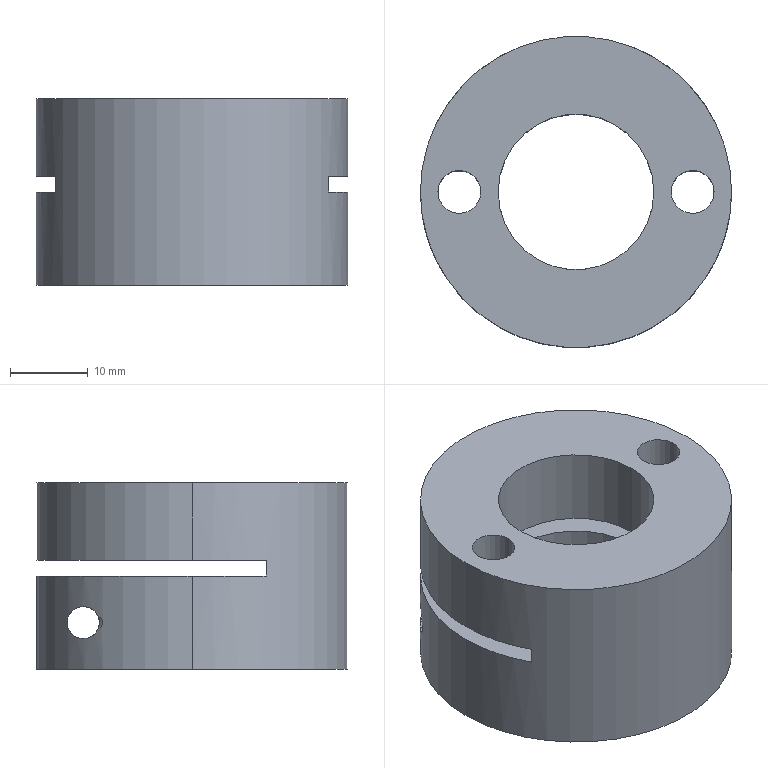Part | NX | features A0001 2 | 1 solid | 39 faces | box 40 x 40 x 24 mm | volume 19127 mm3 | cylinder 22 | plane 14 | cone 3 | commonest cylinder face diameters 5.5 x8 20 x4 40 x4 4.134 x2 5.6 x2 9 x2
STEP:
#1=CARTESIAN_POINT('',(-67.75,25.,-12.));
#2=VERTEX_POINT('',#1);
#3=CARTESIAN_POINT('',(-62.25,25.,-12.));
#4=VERTEX_POINT('',#3);
#5=CARTESIAN_POINT('',(-65.,25.,-12.));
#6=DIRECTION('',(0.,0.,-1.));
#7=DIRECTION('',(-1.,0.,0.));
#8=AXIS2_PLACEMENT_3D('',#5,#6,#7);
#9=CIRCLE('',#8,2.75);
#10=EDGE_CURVE('',#2,#4,#9,.T.);
#11=ORIENTED_EDGE('',*,*,#10,.F.);
#12=CARTESIAN_POINT('',(-67.75,25.,-22.));
#13=VERTEX_POINT('',#12);
#14=CARTESIAN_POINT('',(-67.75,25.,-22.));
#15=DIRECTION('',(0.,0.,1.));
#16=VECTOR('',#15,1000.);
#17=LINE('',#14,#16);
#18=EDGE_CURVE('',#2,#13,#17,.F.);
#19=ORIENTED_EDGE('',*,*,#18,.T.);
#20=CARTESIAN_POINT('',(-62.25,25.,-22.));
#21=VERTEX_POINT('',#20);
#22=CARTESIAN_POINT('',(-65.,25.,-22.));
#23=DIRECTION('',(0.,0.,1.));
#24=DIRECTION('',(1.,0.,0.));
#25=AXIS2_PLACEMENT_3D('',#22,#23,#24);
#26=CIRCLE('',#25,2.75);
#27=EDGE_CURVE('',#21,#13,#26,.T.);
#28=ORIENTED_EDGE('',*,*,#27,.F.);
#29=CARTESIAN_POINT('',(-62.25,25.,-22.));
#30=DIRECTION('',(0.,0.,1.));
#31=VECTOR('',#30,1000.);
#32=LINE('',#29,#31);
#33=EDGE_CURVE('',#21,#4,#32,.T.);
#34=ORIENTED_EDGE('',*,*,#33,.T.);
#35=EDGE_LOOP('',(#11,#19,#28,#34));
#36=FACE_BOUND('',#35,.T.);
#37=CARTESIAN_POINT('',(-65.,25.,-12.));
#38=DIRECTION('',(0.,0.,-1.));
#39=DIRECTION('',(-1.,0.,0.));
#40=AXIS2_PLACEMENT_3D('',#37,#38,#39);
#41=CYLINDRICAL_SURFACE('',#40,2.75);
#42=ADVANCED_FACE('',(#36),#41,.F.);
#43=ORIENTED_EDGE('',*,*,#33,.F.);
#44=CARTESIAN_POINT('',(-65.,25.,-22.));
#45=DIRECTION('',(0.,0.,1.));
#46=DIRECTION('',(-1.,0.,0.));
#47=AXIS2_PLACEMENT_3D('',#44,#45,#46);
#48=CIRCLE('',#47,2.75);
#49=EDGE_CURVE('',#13,#21,#48,.T.);
#50=ORIENTED_EDGE('',*,*,#49,.F.);
#51=ORIENTED_EDGE('',*,*,#18,.F.);
#52=CARTESIAN_POINT('',(-65.,25.,-12.));
#53=DIRECTION('',(0.,0.,-1.));
#54=DIRECTION('',(1.,0.,0.));
#55=AXIS2_PLACEMENT_3D('',#52,#53,#54);
#56=CIRCLE('',#55,2.75);
#57=EDGE_CURVE('',#4,#2,#56,.T.);
#58=ORIENTED_EDGE('',*,*,#57,.F.);
#59=EDGE_LOOP('',(#43,#50,#51,#58));
#60=FACE_BOUND('',#59,.T.);
#61=CARTESIAN_POINT('',(-65.,25.,-12.));
#62=DIRECTION('',(0.,0.,-1.));
#63=DIRECTION('',(-1.,0.,0.));
#64=AXIS2_PLACEMENT_3D('',#61,#62,#63);
#65=CYLINDRICAL_SURFACE('',#64,2.75);
#66=ADVANCED_FACE('',(#60),#65,.F.);
#67=CARTESIAN_POINT('',(-80.75,39.,-27.5));
#68=VERTEX_POINT('',#67);
#69=CARTESIAN_POINT('',(-81.183,39.,-27.933));
#70=VERTEX_POINT('',#69);
#71=CARTESIAN_POINT('',(-80.75,39.,-27.5));
#72=DIRECTION('',(-0.7071,0.,-0.7071));
#73=VECTOR('',#72,1000.);
#74=LINE('',#71,#73);
#75=EDGE_CURVE('',#68,#70,#74,.T.);
#76=ORIENTED_EDGE('',*,*,#75,.F.);
#77=CARTESIAN_POINT('',(-80.75,39.,-32.5));
#78=VERTEX_POINT('',#77);
#79=CARTESIAN_POINT('',(-80.75,39.,-30.));
#80=DIRECTION('',(-1.,0.,0.));
#81=DIRECTION('',(0.,0.,-1.));
#82=AXIS2_PLACEMENT_3D('',#79,#80,#81);
#83=CIRCLE('',#82,2.5);
#84=EDGE_CURVE('',#78,#68,#83,.T.);
#85=ORIENTED_EDGE('',*,*,#84,.F.);
#86=CARTESIAN_POINT('',(-81.183,39.,-32.067));
#87=VERTEX_POINT('',#86);
#88=CARTESIAN_POINT('',(-80.75,39.,-32.5));
#89=DIRECTION('',(-0.7071,0.,0.7071));
#90=VECTOR('',#89,1000.);
#91=LINE('',#88,#90);
#92=EDGE_CURVE('',#87,#78,#91,.F.);
#93=ORIENTED_EDGE('',*,*,#92,.F.);
#94=CARTESIAN_POINT('',(-81.183,39.,-30.));
#95=DIRECTION('',(-1.,0.,0.));
#96=DIRECTION('',(0.,0.,-1.));
#97=AXIS2_PLACEMENT_3D('',#94,#95,#96);
#98=CIRCLE('',#97,2.067);
#99=EDGE_CURVE('',#87,#70,#98,.T.);
#100=ORIENTED_EDGE('',*,*,#99,.T.);
#101=EDGE_LOOP('',(#76,#85,#93,#100));
#102=FACE_BOUND('',#101,.T.);
#103=CARTESIAN_POINT('',(-81.235,39.,-30.));
#104=DIRECTION('',(1.,0.,0.));
#105=DIRECTION('',(0.,0.,-1.));
#106=AXIS2_PLACEMENT_3D('',#103,#104,#105);
#107=CONICAL_SURFACE('',#106,2.015,0.7854);
#108=ADVANCED_FACE('',(#102),#107,.F.);
#109=CARTESIAN_POINT('',(-81.183,39.,-30.));
#110=DIRECTION('',(-1.,0.,0.));
#111=DIRECTION('',(0.,0.,1.));
#112=AXIS2_PLACEMENT_3D('',#109,#110,#111);
#113=CIRCLE('',#112,2.067);
#114=EDGE_CURVE('',#70,#87,#113,.T.);
#115=ORIENTED_EDGE('',*,*,#114,.T.);
#116=ORIENTED_EDGE('',*,*,#92,.T.);
#117=CARTESIAN_POINT('',(-80.75,39.,-30.));
#118=DIRECTION('',(-1.,0.,0.));
#119=DIRECTION('',(0.,0.,1.));
#120=AXIS2_PLACEMENT_3D('',#117,#118,#119);
#121=CIRCLE('',#120,2.5);
#122=EDGE_CURVE('',#68,#78,#121,.T.);
#123=ORIENTED_EDGE('',*,*,#122,.F.);
#124=ORIENTED_EDGE('',*,*,#75,.T.);
#125=EDGE_LOOP('',(#115,#116,#123,#124));
#126=FACE_BOUND('',#125,.T.);
#127=CARTESIAN_POINT('',(-81.235,39.,-30.));
#128=DIRECTION('',(1.,0.,0.));
#129=DIRECTION('',(0.,0.,-1.));
#130=AXIS2_PLACEMENT_3D('',#127,#128,#129);
#131=CONICAL_SURFACE('',#130,2.015,0.7854);
#132=ADVANCED_FACE('',(#126),#131,.F.);
#133=CARTESIAN_POINT('',(-94.283,39.,-32.067));
#134=VERTEX_POINT('',#133);
#135=CARTESIAN_POINT('',(-94.283,39.,-27.933));
#136=VERTEX_POINT('',#135);
#137=CARTESIAN_POINT('',(-94.283,39.,-32.067));
#138=CARTESIAN_POINT('',(-93.803,39.491,-32.067));
#139=CARTESIAN_POINT('',(-93.042,40.184,-31.817));
#140=CARTESIAN_POINT('',(-92.16,40.884,-31.003));
#141=CARTESIAN_POINT('',(-91.786,41.159,-30.));
#142=CARTESIAN_POINT('',(-92.16,40.884,-28.997));
#143=CARTESIAN_POINT('',(-93.042,40.185,-28.183));
#144=CARTESIAN_POINT('',(-93.803,39.49,-27.933));
#145=CARTESIAN_POINT('',(-94.283,39.,-27.933));
#146=B_SPLINE_CURVE_WITH_KNOTS('',3,(#137,#138,#139,#140,#141,#142,#143,#144,#145),.UNSPECIFIED.,.F.,.F.,(4,1,1,1,1,1,4),(0.,0.25,0.375,0.5,0.625,0.75,1.),.UNSPECIFIED.);
#147=EDGE_CURVE('',#134,#136,#146,.T.);
#148=ORIENTED_EDGE('',*,*,#147,.F.);
#149=CARTESIAN_POINT('',(-81.183,39.,-32.067));
#150=DIRECTION('',(-1.,0.,0.));
#151=VECTOR('',#150,1000.);
#152=LINE('',#149,#151);
#153=EDGE_CURVE('',#134,#87,#152,.F.);
#154=ORIENTED_EDGE('',*,*,#153,.T.);
#155=ORIENTED_EDGE('',*,*,#114,.F.);
#156=CARTESIAN_POINT('',(-81.183,39.,-27.933));
#157=DIRECTION('',(-1.,0.,0.));
#158=VECTOR('',#157,1000.);
#159=LINE('',#156,#158);
#160=EDGE_CURVE('',#70,#136,#159,.T.);
#161=ORIENTED_EDGE('',*,*,#160,.T.);
#162=EDGE_LOOP('',(#148,#154,#155,#161));
#163=FACE_BOUND('',#162,.T.);
#164=CARTESIAN_POINT('',(-88.557,39.,-30.));
#165=DIRECTION('',(1.,0.,0.));
#166=DIRECTION('',(0.,0.,-1.));
#167=AXIS2_PLACEMENT_3D('',#164,#165,#166);
#168=CYLINDRICAL_SURFACE('',#167,2.067);
#169=ADVANCED_FACE('',(#163),#168,.F.);
#170=CARTESIAN_POINT('',(-95.93,37.093,-30.797));
#171=VERTEX_POINT('',#170);
#172=CARTESIAN_POINT('',(-95.93,37.093,-29.203));
#173=VERTEX_POINT('',#172);
#174=CARTESIAN_POINT('',(-95.93,37.093,-30.797));
#175=CARTESIAN_POINT('',(-96.04,36.948,-30.735));
#176=CARTESIAN_POINT('',(-96.249,36.663,-30.559));
#177=CARTESIAN_POINT('',(-96.42,36.419,-30.));
#178=CARTESIAN_POINT('',(-96.249,36.663,-29.441));
#179=CARTESIAN_POINT('',(-96.04,36.948,-29.265));
#180=CARTESIAN_POINT('',(-95.93,37.093,-29.203));
#181=B_SPLINE_CURVE_WITH_KNOTS('',3,(#174,#175,#176,#177,#178,#179,#180),.UNSPECIFIED.,.F.,.F.,(4,1,1,1,4),(0.,0.25,0.5,0.75,1.),.UNSPECIFIED.);
#182=EDGE_CURVE('',#171,#173,#181,.T.);
#183=ORIENTED_EDGE('',*,*,#182,.T.);
#184=CARTESIAN_POINT('',(-95.93,39.,-30.));
#185=DIRECTION('',(1.,0.,0.));
#186=DIRECTION('',(0.,-0.9227,0.3854));
#187=AXIS2_PLACEMENT_3D('',#184,#185,#186);
#188=CIRCLE('',#187,2.067);
#189=EDGE_CURVE('',#173,#171,#188,.T.);
#190=ORIENTED_EDGE('',*,*,#189,.T.);
#191=EDGE_LOOP('',(#183,#190));
#192=FACE_BOUND('',#191,.T.);
#193=CARTESIAN_POINT('',(-95.878,39.,-30.));
#194=DIRECTION('',(-1.,0.,0.));
#195=DIRECTION('',(0.,0.,1.));
#196=AXIS2_PLACEMENT_3D('',#193,#194,#195);
#197=CONICAL_SURFACE('',#196,2.015,0.7854);
#198=ADVANCED_FACE('',(#192),#197,.F.);
#199=ORIENTED_EDGE('',*,*,#160,.F.);
#200=ORIENTED_EDGE('',*,*,#99,.F.);
#201=ORIENTED_EDGE('',*,*,#153,.F.);
#202=CARTESIAN_POINT('',(-95.93,37.093,-30.797));
#203=CARTESIAN_POINT('',(-95.653,37.459,-31.674));
#204=CARTESIAN_POINT('',(-94.972,38.294,-32.067));
#205=CARTESIAN_POINT('',(-94.283,39.,-32.067));
#206=B_SPLINE_CURVE_WITH_KNOTS('',3,(#202,#203,#204,#205),.UNSPECIFIED.,.F.,.F.,(4,4),(0.,1.),.UNSPECIFIED.);
#207=EDGE_CURVE('',#134,#171,#206,.F.);
#208=ORIENTED_EDGE('',*,*,#207,.T.);
#209=ORIENTED_EDGE('',*,*,#189,.F.);
#210=CARTESIAN_POINT('',(-94.283,39.,-27.933));
#211=CARTESIAN_POINT('',(-94.972,38.295,-27.933));
#212=CARTESIAN_POINT('',(-95.653,37.459,-28.326));
#213=CARTESIAN_POINT('',(-95.93,37.093,-29.203));
#214=B_SPLINE_CURVE_WITH_KNOTS('',3,(#210,#211,#212,#213),.UNSPECIFIED.,.F.,.F.,(4,4),(0.,1.),.UNSPECIFIED.);
#215=EDGE_CURVE('',#173,#136,#214,.F.);
#216=ORIENTED_EDGE('',*,*,#215,.T.);
#217=EDGE_LOOP('',(#199,#200,#201,#208,#209,#216));
#218=FACE_BOUND('',#217,.T.);
#219=CARTESIAN_POINT('',(-88.557,39.,-30.));
#220=DIRECTION('',(1.,0.,0.));
#221=DIRECTION('',(0.,0.,-1.));
#222=AXIS2_PLACEMENT_3D('',#219,#220,#221);
#223=CYLINDRICAL_SURFACE('',#222,2.067);
#224=ADVANCED_FACE('',(#218),#223,.F.);
#225=CARTESIAN_POINT('',(-97.75,25.,-24.));
#226=VERTEX_POINT('',#225);
#227=CARTESIAN_POINT('',(-92.25,25.,-24.));
#228=VERTEX_POINT('',#227);
#229=CARTESIAN_POINT('',(-95.,25.,-24.));
#230=DIRECTION('',(0.,0.,-1.));
#231=DIRECTION('',(-1.,0.,0.));
#232=AXIS2_PLACEMENT_3D('',#229,#230,#231);
#233=CIRCLE('',#232,2.75);
#234=EDGE_CURVE('',#226,#228,#233,.T.);
#235=ORIENTED_EDGE('',*,*,#234,.F.);
#236=CARTESIAN_POINT('',(-97.75,25.,-36.));
#237=VERTEX_POINT('',#236);
#238=CARTESIAN_POINT('',(-97.75,25.,-36.));
#239=DIRECTION('',(0.,0.,1.));
#240=VECTOR('',#239,1000.);
#241=LINE('',#238,#240);
#242=EDGE_CURVE('',#226,#237,#241,.F.);
#243=ORIENTED_EDGE('',*,*,#242,.T.);
#244=CARTESIAN_POINT('',(-92.25,25.,-36.));
#245=VERTEX_POINT('',#244);
#246=CARTESIAN_POINT('',(-95.,25.,-36.));
#247=DIRECTION('',(0.,0.,1.));
#248=DIRECTION('',(1.,0.,0.));
#249=AXIS2_PLACEMENT_3D('',#246,#247,#248);
#250=CIRCLE('',#249,2.75);
#251=EDGE_CURVE('',#245,#237,#250,.T.);
#252=ORIENTED_EDGE('',*,*,#251,.F.);
#253=CARTESIAN_POINT('',(-92.25,25.,-36.));
#254=DIRECTION('',(0.,0.,1.));
#255=VECTOR('',#254,1000.);
#256=LINE('',#253,#255);
#257=EDGE_CURVE('',#245,#228,#256,.T.);
#258=ORIENTED_EDGE('',*,*,#257,.T.);
#259=EDGE_LOOP('',(#235,#243,#252,#258));
#260=FACE_BOUND('',#259,.T.);
#261=CARTESIAN_POINT('',(-95.,25.,-12.));
#262=DIRECTION('',(0.,0.,-1.));
#263=DIRECTION('',(-1.,0.,0.));
#264=AXIS2_PLACEMENT_3D('',#261,#262,#263);
#265=CYLINDRICAL_SURFACE('',#264,2.75);
#266=ADVANCED_FACE('',(#260),#265,.F.);
#267=CARTESIAN_POINT('',(-79.25,10.,-36.));
#268=VERTEX_POINT('',#267);
#269=CARTESIAN_POINT('',(-80.75,10.,-36.));
#270=VERTEX_POINT('',#269);
#271=CARTESIAN_POINT('',(-79.25,10.,-36.));
#272=DIRECTION('',(-1.,0.,0.));
#273=VECTOR('',#272,1000.);
#274=LINE('',#271,#273);
#275=EDGE_CURVE('',#268,#270,#274,.T.);
#276=ORIENTED_EDGE('',*,*,#275,.T.);
#277=CARTESIAN_POINT('',(-80.75,10.,-24.));
#278=VERTEX_POINT('',#277);
#279=CARTESIAN_POINT('',(-80.75,10.,-24.));
#280=DIRECTION('',(0.,0.,-1.));
#281=VECTOR('',#280,1000.);
#282=LINE('',#279,#281);
#283=EDGE_CURVE('',#278,#270,#282,.T.);
#284=ORIENTED_EDGE('',*,*,#283,.F.);
#285=CARTESIAN_POINT('',(-79.25,10.,-24.));
#286=VERTEX_POINT('',#285);
#287=CARTESIAN_POINT('',(-80.75,10.,-24.));
#288=DIRECTION('',(1.,0.,0.));
#289=VECTOR('',#288,1000.);
#290=LINE('',#287,#289);
#291=EDGE_CURVE('',#278,#286,#290,.T.);
#292=ORIENTED_EDGE('',*,*,#291,.T.);
#293=CARTESIAN_POINT('',(-79.25,10.,-36.));
#294=DIRECTION('',(0.,0.,1.));
#295=VECTOR('',#294,1000.);
#296=LINE('',#293,#295);
#297=EDGE_CURVE('',#268,#286,#296,.T.);
#298=ORIENTED_EDGE('',*,*,#297,.F.);
#299=EDGE_LOOP('',(#276,#284,#292,#298));
#300=FACE_BOUND('',#299,.T.);
#301=CARTESIAN_POINT('',(-79.25,10.,-36.));
#302=DIRECTION('',(0.,-1.,0.));
#303=DIRECTION('',(-1.,0.,0.));
#304=AXIS2_PLACEMENT_3D('',#301,#302,#303);
#305=PLANE('',#304);
#306=ADVANCED_FACE('',(#300),#305,.F.);
#307=ORIENTED_EDGE('',*,*,#283,.T.);
#308=CARTESIAN_POINT('',(-80.75,15.028,-36.));
#309=VERTEX_POINT('',#308);
#310=CARTESIAN_POINT('',(-80.75,10.,-36.));
#311=DIRECTION('',(0.,1.,0.));
#312=VECTOR('',#311,1000.);
#313=LINE('',#310,#312);
#314=EDGE_CURVE('',#270,#309,#313,.T.);
#315=ORIENTED_EDGE('',*,*,#314,.T.);
#316=CARTESIAN_POINT('',(-80.75,15.028,-24.));
#317=VERTEX_POINT('',#316);
#318=CARTESIAN_POINT('',(-80.75,15.028,-24.));
#319=DIRECTION('',(0.,0.,-1.));
#320=VECTOR('',#319,1000.);
#321=LINE('',#318,#320);
#322=EDGE_CURVE('',#317,#309,#321,.T.);
#323=ORIENTED_EDGE('',*,*,#322,.F.);
#324=CARTESIAN_POINT('',(-80.75,15.028,-24.));
#325=DIRECTION('',(0.,-1.,0.));
#326=VECTOR('',#325,1000.);
#327=LINE('',#324,#326);
#328=EDGE_CURVE('',#317,#278,#327,.T.);
#329=ORIENTED_EDGE('',*,*,#328,.T.);
#330=EDGE_LOOP('',(#307,#315,#323,#329));
#331=FACE_BOUND('',#330,.T.);
#332=CARTESIAN_POINT('',(-80.75,10.,-36.));
#333=DIRECTION('',(-1.,0.,0.));
#334=DIRECTION('',(0.,0.,1.));
#335=AXIS2_PLACEMENT_3D('',#332,#333,#334);
#336=PLANE('',#335);
#337=ADVANCED_FACE('',(#331),#336,.F.);
#338=CARTESIAN_POINT('',(-79.25,15.028,-24.));
#339=VERTEX_POINT('',#338);
#340=CARTESIAN_POINT('',(-80.,25.,-24.));
#341=DIRECTION('',(0.,0.,1.));
#342=DIRECTION('',(-0.075,-0.9972,0.));
#343=AXIS2_PLACEMENT_3D('',#340,#341,#342);
#344=CIRCLE('',#343,10.);
#345=EDGE_CURVE('',#317,#339,#344,.T.);
#346=ORIENTED_EDGE('',*,*,#345,.T.);
#347=CARTESIAN_POINT('',(-79.25,10.,-24.));
#348=DIRECTION('',(0.,1.,0.));
#349=VECTOR('',#348,1000.);
#350=LINE('',#347,#349);
#351=EDGE_CURVE('',#286,#339,#350,.T.);
#352=ORIENTED_EDGE('',*,*,#351,.F.);
#353=ORIENTED_EDGE('',*,*,#291,.F.);
#354=ORIENTED_EDGE('',*,*,#328,.F.);
#355=EDGE_LOOP('',(#346,#352,#353,#354));
#356=FACE_BOUND('',#355,.T.);
#357=CARTESIAN_POINT('',(-80.,25.,-24.));
#358=DIRECTION('',(0.,0.,-1.));
#359=DIRECTION('',(-1.,0.,0.));
#360=AXIS2_PLACEMENT_3D('',#357,#358,#359);
#361=PLANE('',#360);
#362=ADVANCED_FACE('',(#356),#361,.T.);
#363=ORIENTED_EDGE('',*,*,#297,.T.);
#364=ORIENTED_EDGE('',*,*,#351,.T.);
#365=CARTESIAN_POINT('',(-79.25,15.028,-36.));
#366=VERTEX_POINT('',#365);
#367=CARTESIAN_POINT('',(-79.25,15.028,-36.));
#368=DIRECTION('',(0.,0.,1.));
#369=VECTOR('',#368,1000.);
#370=LINE('',#367,#369);
#371=EDGE_CURVE('',#366,#339,#370,.T.);
#372=ORIENTED_EDGE('',*,*,#371,.F.);
#373=CARTESIAN_POINT('',(-79.25,15.028,-36.));
#374=DIRECTION('',(0.,-1.,0.));
#375=VECTOR('',#374,1000.);
#376=LINE('',#373,#375);
#377=EDGE_CURVE('',#366,#268,#376,.T.);
#378=ORIENTED_EDGE('',*,*,#377,.T.);
#379=EDGE_LOOP('',(#363,#364,#372,#378));
#380=FACE_BOUND('',#379,.T.);
#381=CARTESIAN_POINT('',(-79.25,50.,-36.));
#382=DIRECTION('',(1.,0.,0.));
#383=DIRECTION('',(0.,0.,-1.));
#384=AXIS2_PLACEMENT_3D('',#381,#382,#383);
#385=PLANE('',#384);
#386=ADVANCED_FACE('',(#380),#385,.F.);
#387=CARTESIAN_POINT('',(-62.25,25.,-24.));
#388=VERTEX_POINT('',#387);
#389=CARTESIAN_POINT('',(-62.25,25.,-36.));
#390=VERTEX_POINT('',#389);
#391=CARTESIAN_POINT('',(-62.25,25.,-36.));
#392=DIRECTION('',(0.,0.,1.));
#393=VECTOR('',#392,1000.);
#394=LINE('',#391,#393);
#395=EDGE_CURVE('',#388,#390,#394,.F.);
#396=ORIENTED_EDGE('',*,*,#395,.T.);
#397=CARTESIAN_POINT('',(-67.75,25.,-36.));
#398=VERTEX_POINT('',#397);
#399=CARTESIAN_POINT('',(-65.,25.,-36.));
#400=DIRECTION('',(0.,0.,1.));
#401=DIRECTION('',(-1.,0.,0.));
#402=AXIS2_PLACEMENT_3D('',#399,#400,#401);
#403=CIRCLE('',#402,2.75);
#404=EDGE_CURVE('',#398,#390,#403,.T.);
#405=ORIENTED_EDGE('',*,*,#404,.F.);
#406=CARTESIAN_POINT('',(-67.75,25.,-24.));
#407=VERTEX_POINT('',#406);
#408=CARTESIAN_POINT('',(-67.75,25.,-36.));
#409=DIRECTION('',(0.,0.,1.));
#410=VECTOR('',#409,1000.);
#411=LINE('',#408,#410);
#412=EDGE_CURVE('',#398,#407,#411,.T.);
#413=ORIENTED_EDGE('',*,*,#412,.T.);
#414=CARTESIAN_POINT('',(-65.,25.,-24.));
#415=DIRECTION('',(0.,0.,-1.));
#416=DIRECTION('',(1.,0.,0.));
#417=AXIS2_PLACEMENT_3D('',#414,#415,#416);
#418=CIRCLE('',#417,2.75);
#419=EDGE_CURVE('',#388,#407,#418,.T.);
#420=ORIENTED_EDGE('',*,*,#419,.F.);
#421=EDGE_LOOP('',(#396,#405,#413,#420));
#422=FACE_BOUND('',#421,.T.);
#423=CARTESIAN_POINT('',(-65.,25.,-12.));
#424=DIRECTION('',(0.,0.,-1.));
#425=DIRECTION('',(-1.,0.,0.));
#426=AXIS2_PLACEMENT_3D('',#423,#424,#425);
#427=CYLINDRICAL_SURFACE('',#426,2.75);
#428=ADVANCED_FACE('',(#422),#427,.F.);
#429=CARTESIAN_POINT('',(-65.,25.,-24.));
#430=DIRECTION('',(0.,0.,-1.));
#431=DIRECTION('',(-1.,0.,0.));
#432=AXIS2_PLACEMENT_3D('',#429,#430,#431);
#433=CIRCLE('',#432,2.75);
#434=EDGE_CURVE('',#407,#388,#433,.T.);
#435=ORIENTED_EDGE('',*,*,#434,.F.);
#436=ORIENTED_EDGE('',*,*,#412,.F.);
#437=CARTESIAN_POINT('',(-65.,25.,-36.));
#438=DIRECTION('',(0.,0.,1.));
#439=DIRECTION('',(1.,0.,0.));
#440=AXIS2_PLACEMENT_3D('',#437,#438,#439);
#441=CIRCLE('',#440,2.75);
#442=EDGE_CURVE('',#390,#398,#441,.T.);
#443=ORIENTED_EDGE('',*,*,#442,.F.);
#444=ORIENTED_EDGE('',*,*,#395,.F.);
#445=EDGE_LOOP('',(#435,#436,#443,#444));
#446=FACE_BOUND('',#445,.T.);
#447=CARTESIAN_POINT('',(-65.,25.,-12.));
#448=DIRECTION('',(0.,0.,-1.));
#449=DIRECTION('',(-1.,0.,0.));
#450=AXIS2_PLACEMENT_3D('',#447,#448,#449);
#451=CYLINDRICAL_SURFACE('',#450,2.75);
#452=ADVANCED_FACE('',(#446),#451,.F.);
#453=CARTESIAN_POINT('',(-62.4,15.5,-24.));
#454=VERTEX_POINT('',#453);
#455=CARTESIAN_POINT('',(-62.4,15.5,-22.));
#456=VERTEX_POINT('',#455);
#457=CARTESIAN_POINT('',(-62.4,15.5,-24.));
#458=DIRECTION('',(0.,0.,1.));
#459=VECTOR('',#458,1000.);
#460=LINE('',#457,#459);
#461=EDGE_CURVE('',#454,#456,#460,.T.);
#462=ORIENTED_EDGE('',*,*,#461,.F.);
#463=CARTESIAN_POINT('',(-76.878,15.5,-24.));
#464=VERTEX_POINT('',#463);
#465=CARTESIAN_POINT('',(-62.4,15.5,-24.));
#466=DIRECTION('',(-1.,0.,0.));
#467=VECTOR('',#466,1000.);
#468=LINE('',#465,#467);
#469=EDGE_CURVE('',#454,#464,#468,.T.);
#470=ORIENTED_EDGE('',*,*,#469,.T.);
#471=CARTESIAN_POINT('',(-76.878,15.5,-22.));
#472=VERTEX_POINT('',#471);
#473=CARTESIAN_POINT('',(-76.878,15.5,-22.));
#474=DIRECTION('',(0.,0.,-1.));
#475=VECTOR('',#474,1000.);
#476=LINE('',#473,#475);
#477=EDGE_CURVE('',#472,#464,#476,.T.);
#478=ORIENTED_EDGE('',*,*,#477,.F.);
#479=CARTESIAN_POINT('',(-62.4,15.5,-22.));
#480=DIRECTION('',(-1.,0.,0.));
#481=VECTOR('',#480,1000.);
#482=LINE('',#479,#481);
#483=EDGE_CURVE('',#456,#472,#482,.T.);
#484=ORIENTED_EDGE('',*,*,#483,.F.);
#485=EDGE_LOOP('',(#462,#470,#478,#484));
#486=FACE_BOUND('',#485,.T.);
#487=CARTESIAN_POINT('',(-60.,15.5,-22.));
#488=DIRECTION('',(0.,-1.,0.));
#489=DIRECTION('',(-1.,0.,0.));
#490=AXIS2_PLACEMENT_3D('',#487,#488,#489);
#491=PLANE('',#490);
#492=ADVANCED_FACE('',(#486),#491,.F.);
#493=CARTESIAN_POINT('',(-74.,39.,-32.8));
#494=VERTEX_POINT('',#493);
#495=CARTESIAN_POINT('',(-79.25,39.,-32.8));
#496=VERTEX_POINT('',#495);
#497=CARTESIAN_POINT('',(-79.25,39.,-32.8));
#498=DIRECTION('',(1.,0.,0.));
#499=VECTOR('',#498,1000.);
#500=LINE('',#497,#499);
#501=EDGE_CURVE('',#494,#496,#500,.F.);
#502=ORIENTED_EDGE('',*,*,#501,.T.);
#503=CARTESIAN_POINT('',(-79.25,39.,-27.2));
#504=VERTEX_POINT('',#503);
#505=CARTESIAN_POINT('',(-79.25,39.,-30.));
#506=DIRECTION('',(1.,0.,0.));
#507=DIRECTION('',(0.,0.,1.));
#508=AXIS2_PLACEMENT_3D('',#505,#506,#507);
#509=CIRCLE('',#508,2.8);
#510=EDGE_CURVE('',#504,#496,#509,.T.);
#511=ORIENTED_EDGE('',*,*,#510,.F.);
#512=CARTESIAN_POINT('',(-74.,39.,-27.2));
#513=VERTEX_POINT('',#512);
#514=CARTESIAN_POINT('',(-79.25,39.,-27.2));
#515=DIRECTION('',(1.,0.,0.));
#516=VECTOR('',#515,1000.);
#517=LINE('',#514,#516);
#518=EDGE_CURVE('',#504,#513,#517,.T.);
#519=ORIENTED_EDGE('',*,*,#518,.T.);
#520=CARTESIAN_POINT('',(-74.,39.,-30.));
#521=DIRECTION('',(-1.,0.,0.));
#522=DIRECTION('',(0.,0.,-1.));
#523=AXIS2_PLACEMENT_3D('',#520,#521,#522);
#524=CIRCLE('',#523,2.8);
#525=EDGE_CURVE('',#494,#513,#524,.T.);
#526=ORIENTED_EDGE('',*,*,#525,.F.);
#527=EDGE_LOOP('',(#502,#511,#519,#526));
#528=FACE_BOUND('',#527,.T.);
#529=CARTESIAN_POINT('',(-76.625,39.,-30.));
#530=DIRECTION('',(-1.,0.,0.));
#531=DIRECTION('',(0.,0.,1.));
#532=AXIS2_PLACEMENT_3D('',#529,#530,#531);
#533=CYLINDRICAL_SURFACE('',#532,2.8);
#534=ADVANCED_FACE('',(#528),#533,.F.);
#535=CARTESIAN_POINT('',(-74.,39.,-30.));
#536=DIRECTION('',(-1.,0.,0.));
#537=DIRECTION('',(0.,0.,1.));
#538=AXIS2_PLACEMENT_3D('',#535,#536,#537);
#539=CIRCLE('',#538,2.8);
#540=EDGE_CURVE('',#513,#494,#539,.T.);
#541=ORIENTED_EDGE('',*,*,#540,.F.);
#542=ORIENTED_EDGE('',*,*,#518,.F.);
#543=CARTESIAN_POINT('',(-79.25,39.,-30.));
#544=DIRECTION('',(1.,0.,0.));
#545=DIRECTION('',(0.,0.,-1.));
#546=AXIS2_PLACEMENT_3D('',#543,#544,#545);
#547=CIRCLE('',#546,2.8);
#548=EDGE_CURVE('',#496,#504,#547,.T.);
#549=ORIENTED_EDGE('',*,*,#548,.F.);
#550=ORIENTED_EDGE('',*,*,#501,.F.);
#551=EDGE_LOOP('',(#541,#542,#549,#550));
#552=FACE_BOUND('',#551,.T.);
#553=CARTESIAN_POINT('',(-76.625,39.,-30.));
#554=DIRECTION('',(-1.,0.,0.));
#555=DIRECTION('',(0.,0.,1.));
#556=AXIS2_PLACEMENT_3D('',#553,#554,#555);
#557=CYLINDRICAL_SURFACE('',#556,2.8);
#558=ADVANCED_FACE('',(#552),#557,.F.);
#559=ORIENTED_EDGE('',*,*,#525,.T.);
#560=ORIENTED_EDGE('',*,*,#540,.T.);
#561=EDGE_LOOP('',(#559,#560));
#562=FACE_BOUND('',#561,.T.);
#563=CARTESIAN_POINT('',(-74.,39.,-34.5));
#564=VERTEX_POINT('',#563);
#565=CARTESIAN_POINT('',(-74.,39.,-25.5));
#566=VERTEX_POINT('',#565);
#567=CARTESIAN_POINT('',(-74.,39.,-30.));
#568=DIRECTION('',(1.,0.,0.));
#569=DIRECTION('',(0.,0.,-1.));
#570=AXIS2_PLACEMENT_3D('',#567,#568,#569);
#571=CIRCLE('',#570,4.5);
#572=EDGE_CURVE('',#564,#566,#571,.T.);
#573=ORIENTED_EDGE('',*,*,#572,.T.);
#574=CARTESIAN_POINT('',(-74.,39.,-30.));
#575=DIRECTION('',(1.,0.,0.));
#576=DIRECTION('',(0.,0.,1.));
#577=AXIS2_PLACEMENT_3D('',#574,#575,#576);
#578=CIRCLE('',#577,4.5);
#579=EDGE_CURVE('',#566,#564,#578,.T.);
#580=ORIENTED_EDGE('',*,*,#579,.T.);
#581=EDGE_LOOP('',(#573,#580));
#582=FACE_BOUND('',#581,.T.);
#583=CARTESIAN_POINT('',(-74.,42.65,-30.));
#584=DIRECTION('',(-1.,0.,0.));
#585=DIRECTION('',(0.,1.,0.));
#586=AXIS2_PLACEMENT_3D('',#583,#584,#585);
#587=PLANE('',#586);
#588=ADVANCED_FACE('',(#562,#582),#587,.F.);
#589=CARTESIAN_POINT('',(-65.717,39.,-34.5));
#590=VERTEX_POINT('',#589);
#591=CARTESIAN_POINT('',(-74.,39.,-34.5));
#592=DIRECTION('',(1.,0.,0.));
#593=VECTOR('',#592,1000.);
#594=LINE('',#591,#593);
#595=EDGE_CURVE('',#564,#590,#594,.T.);
#596=ORIENTED_EDGE('',*,*,#595,.F.);
#597=ORIENTED_EDGE('',*,*,#579,.F.);
#598=CARTESIAN_POINT('',(-65.717,39.,-25.5));
#599=VERTEX_POINT('',#598);
#600=CARTESIAN_POINT('',(-74.,39.,-25.5));
#601=DIRECTION('',(1.,0.,0.));
#602=VECTOR('',#601,1000.);
#603=LINE('',#600,#602);
#604=EDGE_CURVE('',#599,#566,#603,.F.);
#605=ORIENTED_EDGE('',*,*,#604,.F.);
#606=CARTESIAN_POINT('',(-65.717,39.,-34.5));
#607=CARTESIAN_POINT('',(-64.782,38.047,-34.5));
#608=CARTESIAN_POINT('',(-63.51,36.411,-34.028));
#609=CARTESIAN_POINT('',(-62.562,34.808,-32.003));
#610=CARTESIAN_POINT('',(-62.319,34.346,-30.));
#611=CARTESIAN_POINT('',(-62.562,34.808,-27.997));
#612=CARTESIAN_POINT('',(-63.51,36.411,-25.972));
#613=CARTESIAN_POINT('',(-64.782,38.047,-25.5));
#614=CARTESIAN_POINT('',(-65.717,39.,-25.5));
#615=B_SPLINE_CURVE_WITH_KNOTS('',3,(#606,#607,#608,#609,#610,#611,#612,#613,#614),.UNSPECIFIED.,.F.,.F.,(4,1,1,1,1,1,4),(0.,0.25,0.375,0.5,0.625,0.75,1.),.UNSPECIFIED.);
#616=EDGE_CURVE('',#599,#590,#615,.F.);
#617=ORIENTED_EDGE('',*,*,#616,.T.);
#618=EDGE_LOOP('',(#596,#597,#605,#617));
#619=FACE_BOUND('',#618,.T.);
#620=CARTESIAN_POINT('',(-66.625,39.,-30.));
#621=DIRECTION('',(-1.,0.,0.));
#622=DIRECTION('',(0.,0.,1.));
#623=AXIS2_PLACEMENT_3D('',#620,#621,#622);
#624=CYLINDRICAL_SURFACE('',#623,4.5);
#625=ADVANCED_FACE('',(#619),#624,.F.);
#626=CARTESIAN_POINT('',(-65.717,39.,-25.5));
#627=CARTESIAN_POINT('',(-66.296,39.59,-25.5));
#628=CARTESIAN_POINT('',(-67.523,40.694,-25.729));
#629=CARTESIAN_POINT('',(-69.446,42.039,-26.561));
#630=CARTESIAN_POINT('',(-71.025,42.894,-27.616));
#631=CARTESIAN_POINT('',(-72.103,43.378,-28.784));
#632=CARTESIAN_POINT('',(-72.547,43.561,-30.));
#633=CARTESIAN_POINT('',(-72.102,43.378,-31.215));
#634=CARTESIAN_POINT('',(-71.025,42.894,-32.384));
#635=CARTESIAN_POINT('',(-69.446,42.039,-33.439));
#636=CARTESIAN_POINT('',(-67.523,40.694,-34.271));
#637=CARTESIAN_POINT('',(-66.296,39.59,-34.5));
#638=CARTESIAN_POINT('',(-65.717,39.,-34.5));
#639=B_SPLINE_CURVE_WITH_KNOTS('',3,(#626,#627,#628,#629,#630,#631,#632,#633,#634,#635,#636,#637,#638),.UNSPECIFIED.,.F.,.F.,(4,1,1,1,1,1,1,1,1,1,4),(0.,0.125,0.25,0.375,0.4375,0.5,0.5625,0.625,0.75,0.875,1.),.UNSPECIFIED.);
#640=EDGE_CURVE('',#590,#599,#639,.F.);
#641=ORIENTED_EDGE('',*,*,#640,.T.);
#642=ORIENTED_EDGE('',*,*,#604,.T.);
#643=ORIENTED_EDGE('',*,*,#572,.F.);
#644=ORIENTED_EDGE('',*,*,#595,.T.);
#645=EDGE_LOOP('',(#641,#642,#643,#644));
#646=FACE_BOUND('',#645,.T.);
#647=CARTESIAN_POINT('',(-66.625,39.,-30.));
#648=DIRECTION('',(-1.,0.,0.));
#649=DIRECTION('',(0.,0.,1.));
#650=AXIS2_PLACEMENT_3D('',#647,#648,#649);
#651=CYLINDRICAL_SURFACE('',#650,4.5);
#652=ADVANCED_FACE('',(#646),#651,.F.);
#653=ORIENTED_EDGE('',*,*,#616,.F.);
#654=ORIENTED_EDGE('',*,*,#640,.F.);
#655=EDGE_LOOP('',(#653,#654));
#656=FACE_BOUND('',#655,.T.);
#657=CARTESIAN_POINT('',(-60.,25.,-36.));
#658=VERTEX_POINT('',#657);
#659=CARTESIAN_POINT('',(-60.,25.,-24.));
#660=VERTEX_POINT('',#659);
#661=CARTESIAN_POINT('',(-60.,25.,-36.));
#662=DIRECTION('',(0.,0.,1.));
#663=VECTOR('',#662,1000.);
#664=LINE('',#661,#663);
#665=EDGE_CURVE('',#658,#660,#664,.T.);
#666=ORIENTED_EDGE('',*,*,#665,.F.);
#667=CARTESIAN_POINT('',(-79.25,44.986,-36.));
#668=VERTEX_POINT('',#667);
#669=CARTESIAN_POINT('',(-80.,25.,-36.));
#670=DIRECTION('',(0.,0.,-1.));
#671=DIRECTION('',(0.0375,0.9993,0.));
#672=AXIS2_PLACEMENT_3D('',#669,#670,#671);
#673=CIRCLE('',#672,20.);
#674=EDGE_CURVE('',#668,#658,#673,.T.);
#675=ORIENTED_EDGE('',*,*,#674,.F.);
#676=CARTESIAN_POINT('',(-79.25,44.986,-24.));
#677=VERTEX_POINT('',#676);
#678=CARTESIAN_POINT('',(-79.25,44.986,-36.));
#679=DIRECTION('',(0.,0.,1.));
#680=VECTOR('',#679,1000.);
#681=LINE('',#678,#680);
#682=EDGE_CURVE('',#668,#677,#681,.T.);
#683=ORIENTED_EDGE('',*,*,#682,.T.);
#684=CARTESIAN_POINT('',(-80.,25.,-24.));
#685=DIRECTION('',(0.,0.,1.));
#686=DIRECTION('',(1.,0.,0.));
#687=AXIS2_PLACEMENT_3D('',#684,#685,#686);
#688=CIRCLE('',#687,20.);
#689=EDGE_CURVE('',#660,#677,#688,.T.);
#690=ORIENTED_EDGE('',*,*,#689,.F.);
#691=EDGE_LOOP('',(#666,#675,#683,#690));
#692=FACE_BOUND('',#691,.T.);
#693=CARTESIAN_POINT('',(-80.,25.,-24.));
#694=DIRECTION('',(0.,0.,-1.));
#695=DIRECTION('',(-1.,0.,0.));
#696=AXIS2_PLACEMENT_3D('',#693,#694,#695);
#697=CYLINDRICAL_SURFACE('',#696,20.);
#698=ADVANCED_FACE('',(#656,#692),#697,.T.);
#699=CARTESIAN_POINT('',(-79.25,34.972,-24.));
#700=VERTEX_POINT('',#699);
#701=CARTESIAN_POINT('',(-70.,25.,-24.));
#702=VERTEX_POINT('',#701);
#703=CARTESIAN_POINT('',(-80.,25.,-24.));
#704=DIRECTION('',(0.,0.,-1.));
#705=DIRECTION('',(0.075,0.9972,0.));
#706=AXIS2_PLACEMENT_3D('',#703,#704,#705);
#707=CIRCLE('',#706,10.);
#708=EDGE_CURVE('',#700,#702,#707,.T.);
#709=ORIENTED_EDGE('',*,*,#708,.F.);
#710=CARTESIAN_POINT('',(-79.25,34.972,-36.));
#711=VERTEX_POINT('',#710);
#712=CARTESIAN_POINT('',(-79.25,34.972,-24.));
#713=DIRECTION('',(0.,0.,-1.));
#714=VECTOR('',#713,1000.);
#715=LINE('',#712,#714);
#716=EDGE_CURVE('',#700,#711,#715,.T.);
#717=ORIENTED_EDGE('',*,*,#716,.T.);
#718=CARTESIAN_POINT('',(-70.,25.,-36.));
#719=VERTEX_POINT('',#718);
#720=CARTESIAN_POINT('',(-80.,25.,-36.));
#721=DIRECTION('',(0.,0.,1.));
#722=DIRECTION('',(1.,0.,0.));
#723=AXIS2_PLACEMENT_3D('',#720,#721,#722);
#724=CIRCLE('',#723,10.);
#725=EDGE_CURVE('',#719,#711,#724,.T.);
#726=ORIENTED_EDGE('',*,*,#725,.F.);
#727=CARTESIAN_POINT('',(-70.,25.,-36.));
#728=DIRECTION('',(0.,0.,1.));
#729=VECTOR('',#728,1000.);
#730=LINE('',#727,#729);
#731=EDGE_CURVE('',#719,#702,#730,.T.);
#732=ORIENTED_EDGE('',*,*,#731,.T.);
#733=EDGE_LOOP('',(#709,#717,#726,#732));
#734=FACE_BOUND('',#733,.T.);
#735=CARTESIAN_POINT('',(-80.,25.,-20.));
#736=DIRECTION('',(0.,0.,-1.));
#737=DIRECTION('',(-1.,0.,0.));
#738=AXIS2_PLACEMENT_3D('',#735,#736,#737);
#739=CYLINDRICAL_SURFACE('',#738,10.);
#740=ADVANCED_FACE('',(#734),#739,.F.);
#741=ORIENTED_EDGE('',*,*,#419,.T.);
#742=ORIENTED_EDGE('',*,*,#434,.T.);
#743=EDGE_LOOP('',(#741,#742));
#744=FACE_BOUND('',#743,.T.);
#745=CARTESIAN_POINT('',(-80.,25.,-24.));
#746=DIRECTION('',(0.,0.,-1.));
#747=DIRECTION('',(1.,0.,0.));
#748=AXIS2_PLACEMENT_3D('',#745,#746,#747);
#749=CIRCLE('',#748,10.);
#750=EDGE_CURVE('',#702,#464,#749,.T.);
#751=ORIENTED_EDGE('',*,*,#750,.T.);
#752=ORIENTED_EDGE('',*,*,#469,.F.);
#753=CARTESIAN_POINT('',(-80.,25.,-24.));
#754=DIRECTION('',(0.,0.,1.));
#755=DIRECTION('',(0.88,-0.475,0.));
#756=AXIS2_PLACEMENT_3D('',#753,#754,#755);
#757=CIRCLE('',#756,20.);
#758=EDGE_CURVE('',#454,#660,#757,.T.);
#759=ORIENTED_EDGE('',*,*,#758,.T.);
#760=ORIENTED_EDGE('',*,*,#689,.T.);
#761=CARTESIAN_POINT('',(-79.25,44.986,-24.));
#762=DIRECTION('',(0.,-1.,0.));
#763=VECTOR('',#762,1000.);
#764=LINE('',#761,#763);
#765=EDGE_CURVE('',#677,#700,#764,.T.);
#766=ORIENTED_EDGE('',*,*,#765,.T.);
#767=ORIENTED_EDGE('',*,*,#708,.T.);
#768=EDGE_LOOP('',(#751,#752,#759,#760,#766,#767));
#769=FACE_BOUND('',#768,.T.);
#770=CARTESIAN_POINT('',(-60.,15.5,-24.));
#771=DIRECTION('',(0.,0.,-1.));
#772=DIRECTION('',(-1.,0.,0.));
#773=AXIS2_PLACEMENT_3D('',#770,#771,#772);
#774=PLANE('',#773);
#775=ADVANCED_FACE('',(#744,#769),#774,.F.);
#776=ORIENTED_EDGE('',*,*,#510,.T.);
#777=ORIENTED_EDGE('',*,*,#548,.T.);
#778=EDGE_LOOP('',(#776,#777));
#779=FACE_BOUND('',#778,.T.);
#780=ORIENTED_EDGE('',*,*,#682,.F.);
#781=CARTESIAN_POINT('',(-79.25,44.986,-36.));
#782=DIRECTION('',(0.,-1.,0.));
#783=VECTOR('',#782,1000.);
#784=LINE('',#781,#783);
#785=EDGE_CURVE('',#668,#711,#784,.T.);
#786=ORIENTED_EDGE('',*,*,#785,.T.);
#787=ORIENTED_EDGE('',*,*,#716,.F.);
#788=ORIENTED_EDGE('',*,*,#765,.F.);
#789=EDGE_LOOP('',(#780,#786,#787,#788));
#790=FACE_BOUND('',#789,.T.);
#791=CARTESIAN_POINT('',(-79.25,50.,-36.));
#792=DIRECTION('',(1.,0.,0.));
#793=DIRECTION('',(0.,0.,-1.));
#794=AXIS2_PLACEMENT_3D('',#791,#792,#793);
#795=PLANE('',#794);
#796=ADVANCED_FACE('',(#779,#790),#795,.F.);
#797=ORIENTED_EDGE('',*,*,#404,.T.);
#798=ORIENTED_EDGE('',*,*,#442,.T.);
#799=EDGE_LOOP('',(#797,#798));
#800=FACE_BOUND('',#799,.T.);
#801=CARTESIAN_POINT('',(-95.,25.,-36.));
#802=DIRECTION('',(0.,0.,1.));
#803=DIRECTION('',(-1.,0.,0.));
#804=AXIS2_PLACEMENT_3D('',#801,#802,#803);
#805=CIRCLE('',#804,2.75);
#806=EDGE_CURVE('',#237,#245,#805,.T.);
#807=ORIENTED_EDGE('',*,*,#806,.T.);
#808=ORIENTED_EDGE('',*,*,#251,.T.);
#809=EDGE_LOOP('',(#807,#808));
#810=FACE_BOUND('',#809,.T.);
#811=ORIENTED_EDGE('',*,*,#674,.T.);
#812=CARTESIAN_POINT('',(-100.,25.,-36.));
#813=VERTEX_POINT('',#812);
#814=CARTESIAN_POINT('',(-80.,25.,-36.));
#815=DIRECTION('',(0.,0.,-1.));
#816=DIRECTION('',(1.,0.,0.));
#817=AXIS2_PLACEMENT_3D('',#814,#815,#816);
#818=CIRCLE('',#817,20.);
#819=EDGE_CURVE('',#658,#813,#818,.T.);
#820=ORIENTED_EDGE('',*,*,#819,.T.);
#821=CARTESIAN_POINT('',(-80.75,44.986,-36.));
#822=VERTEX_POINT('',#821);
#823=CARTESIAN_POINT('',(-80.,25.,-36.));
#824=DIRECTION('',(0.,0.,-1.));
#825=DIRECTION('',(-1.,0.,0.));
#826=AXIS2_PLACEMENT_3D('',#823,#824,#825);
#827=CIRCLE('',#826,20.);
#828=EDGE_CURVE('',#813,#822,#827,.T.);
#829=ORIENTED_EDGE('',*,*,#828,.T.);
#830=CARTESIAN_POINT('',(-80.75,34.972,-36.));
#831=VERTEX_POINT('',#830);
#832=CARTESIAN_POINT('',(-80.75,34.972,-36.));
#833=DIRECTION('',(0.,1.,0.));
#834=VECTOR('',#833,1000.);
#835=LINE('',#832,#834);
#836=EDGE_CURVE('',#831,#822,#835,.T.);
#837=ORIENTED_EDGE('',*,*,#836,.F.);
#838=CARTESIAN_POINT('',(-90.,25.,-36.));
#839=VERTEX_POINT('',#838);
#840=CARTESIAN_POINT('',(-80.,25.,-36.));
#841=DIRECTION('',(0.,0.,1.));
#842=DIRECTION('',(-0.075,0.9972,0.));
#843=AXIS2_PLACEMENT_3D('',#840,#841,#842);
#844=CIRCLE('',#843,10.);
#845=EDGE_CURVE('',#831,#839,#844,.T.);
#846=ORIENTED_EDGE('',*,*,#845,.T.);
#847=CARTESIAN_POINT('',(-80.,25.,-36.));
#848=DIRECTION('',(0.,0.,1.));
#849=DIRECTION('',(-1.,0.,0.));
#850=AXIS2_PLACEMENT_3D('',#847,#848,#849);
#851=CIRCLE('',#850,10.);
#852=EDGE_CURVE('',#839,#309,#851,.T.);
#853=ORIENTED_EDGE('',*,*,#852,.T.);
#854=ORIENTED_EDGE('',*,*,#314,.F.);
#855=ORIENTED_EDGE('',*,*,#275,.F.);
#856=ORIENTED_EDGE('',*,*,#377,.F.);
#857=CARTESIAN_POINT('',(-80.,25.,-36.));
#858=DIRECTION('',(0.,0.,1.));
#859=DIRECTION('',(0.075,-0.9972,0.));
#860=AXIS2_PLACEMENT_3D('',#857,#858,#859);
#861=CIRCLE('',#860,10.);
#862=EDGE_CURVE('',#366,#719,#861,.T.);
#863=ORIENTED_EDGE('',*,*,#862,.T.);
#864=ORIENTED_EDGE('',*,*,#725,.T.);
#865=ORIENTED_EDGE('',*,*,#785,.F.);
#866=EDGE_LOOP('',(#811,#820,#829,#837,#846,#853,#854,#855,#856,#863,#864,#865));
#867=FACE_BOUND('',#866,.T.);
#868=CARTESIAN_POINT('',(-80.,40.,-36.));
#869=DIRECTION('',(0.,0.,-1.));
#870=DIRECTION('',(-1.,0.,0.));
#871=AXIS2_PLACEMENT_3D('',#868,#869,#870);
#872=PLANE('',#871);
#873=ADVANCED_FACE('',(#800,#810,#867),#872,.T.);
#874=ORIENTED_EDGE('',*,*,#147,.T.);
#875=ORIENTED_EDGE('',*,*,#215,.F.);
#876=ORIENTED_EDGE('',*,*,#182,.F.);
#877=ORIENTED_EDGE('',*,*,#207,.F.);
#878=EDGE_LOOP('',(#874,#875,#876,#877));
#879=FACE_BOUND('',#878,.T.);
#880=CARTESIAN_POINT('',(-80.75,44.986,-24.));
#881=VERTEX_POINT('',#880);
#882=CARTESIAN_POINT('',(-100.,25.,-24.));
#883=VERTEX_POINT('',#882);
#884=CARTESIAN_POINT('',(-80.,25.,-24.));
#885=DIRECTION('',(0.,0.,1.));
#886=DIRECTION('',(-0.0375,0.9993,0.));
#887=AXIS2_PLACEMENT_3D('',#884,#885,#886);
#888=CIRCLE('',#887,20.);
#889=EDGE_CURVE('',#881,#883,#888,.T.);
#890=ORIENTED_EDGE('',*,*,#889,.F.);
#891=CARTESIAN_POINT('',(-80.75,44.986,-24.));
#892=DIRECTION('',(0.,0.,-1.));
#893=VECTOR('',#892,1000.);
#894=LINE('',#891,#893);
#895=EDGE_CURVE('',#881,#822,#894,.T.);
#896=ORIENTED_EDGE('',*,*,#895,.T.);
#897=ORIENTED_EDGE('',*,*,#828,.F.);
#898=CARTESIAN_POINT('',(-100.,25.,-36.));
#899=DIRECTION('',(0.,0.,1.));
#900=VECTOR('',#899,1000.);
#901=LINE('',#898,#900);
#902=EDGE_CURVE('',#813,#883,#901,.T.);
#903=ORIENTED_EDGE('',*,*,#902,.T.);
#904=EDGE_LOOP('',(#890,#896,#897,#903));
#905=FACE_BOUND('',#904,.T.);
#906=CARTESIAN_POINT('',(-80.,25.,-24.));
#907=DIRECTION('',(0.,0.,-1.));
#908=DIRECTION('',(-1.,0.,0.));
#909=AXIS2_PLACEMENT_3D('',#906,#907,#908);
#910=CYLINDRICAL_SURFACE('',#909,20.);
#911=ADVANCED_FACE('',(#879,#905),#910,.T.);
#912=ORIENTED_EDGE('',*,*,#84,.T.);
#913=ORIENTED_EDGE('',*,*,#122,.T.);
#914=EDGE_LOOP('',(#912,#913));
#915=FACE_BOUND('',#914,.T.);
#916=CARTESIAN_POINT('',(-80.75,34.972,-24.));
#917=VERTEX_POINT('',#916);
#918=CARTESIAN_POINT('',(-80.75,34.972,-36.));
#919=DIRECTION('',(0.,0.,1.));
#920=VECTOR('',#919,1000.);
#921=LINE('',#918,#920);
#922=EDGE_CURVE('',#831,#917,#921,.T.);
#923=ORIENTED_EDGE('',*,*,#922,.F.);
#924=ORIENTED_EDGE('',*,*,#836,.T.);
#925=ORIENTED_EDGE('',*,*,#895,.F.);
#926=CARTESIAN_POINT('',(-80.75,44.986,-24.));
#927=DIRECTION('',(0.,-1.,0.));
#928=VECTOR('',#927,1000.);
#929=LINE('',#926,#928);
#930=EDGE_CURVE('',#881,#917,#929,.T.);
#931=ORIENTED_EDGE('',*,*,#930,.T.);
#932=EDGE_LOOP('',(#923,#924,#925,#931));
#933=FACE_BOUND('',#932,.T.);
#934=CARTESIAN_POINT('',(-80.75,10.,-36.));
#935=DIRECTION('',(-1.,0.,0.));
#936=DIRECTION('',(0.,0.,1.));
#937=AXIS2_PLACEMENT_3D('',#934,#935,#936);
#938=PLANE('',#937);
#939=ADVANCED_FACE('',(#915,#933),#938,.F.);
#940=CARTESIAN_POINT('',(-90.,25.,-24.));
#941=VERTEX_POINT('',#940);
#942=CARTESIAN_POINT('',(-90.,25.,-36.));
#943=DIRECTION('',(0.,0.,1.));
#944=VECTOR('',#943,1000.);
#945=LINE('',#942,#944);
#946=EDGE_CURVE('',#839,#941,#945,.T.);
#947=ORIENTED_EDGE('',*,*,#946,.F.);
#948=ORIENTED_EDGE('',*,*,#845,.F.);
#949=ORIENTED_EDGE('',*,*,#922,.T.);
#950=CARTESIAN_POINT('',(-80.,25.,-24.));
#951=DIRECTION('',(0.,0.,-1.));
#952=DIRECTION('',(-1.,0.,0.));
#953=AXIS2_PLACEMENT_3D('',#950,#951,#952);
#954=CIRCLE('',#953,10.);
#955=EDGE_CURVE('',#941,#917,#954,.T.);
#956=ORIENTED_EDGE('',*,*,#955,.F.);
#957=EDGE_LOOP('',(#947,#948,#949,#956));
#958=FACE_BOUND('',#957,.T.);
#959=CARTESIAN_POINT('',(-80.,25.,-20.));
#960=DIRECTION('',(0.,0.,-1.));
#961=DIRECTION('',(-1.,0.,0.));
#962=AXIS2_PLACEMENT_3D('',#959,#960,#961);
#963=CYLINDRICAL_SURFACE('',#962,10.);
#964=ADVANCED_FACE('',(#958),#963,.F.);
#965=CARTESIAN_POINT('',(-90.,25.,-12.));
#966=VERTEX_POINT('',#965);
#967=CARTESIAN_POINT('',(-70.,25.,-12.));
#968=VERTEX_POINT('',#967);
#969=CARTESIAN_POINT('',(-80.,25.,-12.));
#970=DIRECTION('',(0.,0.,-1.));
#971=DIRECTION('',(-1.,0.,0.));
#972=AXIS2_PLACEMENT_3D('',#969,#970,#971);
#973=CIRCLE('',#972,10.);
#974=EDGE_CURVE('',#966,#968,#973,.T.);
#975=ORIENTED_EDGE('',*,*,#974,.F.);
#976=CARTESIAN_POINT('',(-90.,25.,-22.));
#977=VERTEX_POINT('',#976);
#978=CARTESIAN_POINT('',(-90.,25.,-22.));
#979=DIRECTION('',(0.,0.,1.));
#980=VECTOR('',#979,1000.);
#981=LINE('',#978,#980);
#982=EDGE_CURVE('',#966,#977,#981,.F.);
#983=ORIENTED_EDGE('',*,*,#982,.T.);
#984=CARTESIAN_POINT('',(-70.,25.,-22.));
#985=VERTEX_POINT('',#984);
#986=CARTESIAN_POINT('',(-80.,25.,-22.));
#987=DIRECTION('',(0.,0.,1.));
#988=DIRECTION('',(1.,0.,0.));
#989=AXIS2_PLACEMENT_3D('',#986,#987,#988);
#990=CIRCLE('',#989,10.);
#991=EDGE_CURVE('',#985,#977,#990,.T.);
#992=ORIENTED_EDGE('',*,*,#991,.F.);
#993=CARTESIAN_POINT('',(-70.,25.,-22.));
#994=DIRECTION('',(0.,0.,1.));
#995=VECTOR('',#994,1000.);
#996=LINE('',#993,#995);
#997=EDGE_CURVE('',#985,#968,#996,.T.);
#998=ORIENTED_EDGE('',*,*,#997,.T.);
#999=EDGE_LOOP('',(#975,#983,#992,#998));
#1000=FACE_BOUND('',#999,.T.);
#1001=CARTESIAN_POINT('',(-80.,25.,-20.));
#1002=DIRECTION('',(0.,0.,-1.));
#1003=DIRECTION('',(-1.,0.,0.));
#1004=AXIS2_PLACEMENT_3D('',#1001,#1002,#1003);
#1005=CYLINDRICAL_SURFACE('',#1004,10.);
#1006=ADVANCED_FACE('',(#1000),#1005,.F.);
#1007=ORIENTED_EDGE('',*,*,#997,.F.);
#1008=CARTESIAN_POINT('',(-80.,25.,-22.));
#1009=DIRECTION('',(0.,0.,1.));
#1010=DIRECTION('',(0.3122,-0.95,0.));
#1011=AXIS2_PLACEMENT_3D('',#1008,#1009,#1010);
#1012=CIRCLE('',#1011,10.);
#1013=EDGE_CURVE('',#472,#985,#1012,.T.);
#1014=ORIENTED_EDGE('',*,*,#1013,.F.);
#1015=ORIENTED_EDGE('',*,*,#477,.T.);
#1016=ORIENTED_EDGE('',*,*,#750,.F.);
#1017=ORIENTED_EDGE('',*,*,#731,.F.);
#1018=ORIENTED_EDGE('',*,*,#862,.F.);
#1019=ORIENTED_EDGE('',*,*,#371,.T.);
#1020=ORIENTED_EDGE('',*,*,#345,.F.);
#1021=ORIENTED_EDGE('',*,*,#322,.T.);
#1022=ORIENTED_EDGE('',*,*,#852,.F.);
#1023=ORIENTED_EDGE('',*,*,#946,.T.);
#1024=CARTESIAN_POINT('',(-83.122,15.5,-24.));
#1025=VERTEX_POINT('',#1024);
#1026=CARTESIAN_POINT('',(-80.,25.,-24.));
#1027=DIRECTION('',(0.,0.,-1.));
#1028=DIRECTION('',(-0.3122,-0.95,0.));
#1029=AXIS2_PLACEMENT_3D('',#1026,#1027,#1028);
#1030=CIRCLE('',#1029,10.);
#1031=EDGE_CURVE('',#1025,#941,#1030,.T.);
#1032=ORIENTED_EDGE('',*,*,#1031,.F.);
#1033=CARTESIAN_POINT('',(-83.122,15.5,-22.));
#1034=VERTEX_POINT('',#1033);
#1035=CARTESIAN_POINT('',(-83.122,15.5,-24.));
#1036=DIRECTION('',(0.,0.,1.));
#1037=VECTOR('',#1036,1000.);
#1038=LINE('',#1035,#1037);
#1039=EDGE_CURVE('',#1025,#1034,#1038,.T.);
#1040=ORIENTED_EDGE('',*,*,#1039,.T.);
#1041=CARTESIAN_POINT('',(-80.,25.,-22.));
#1042=DIRECTION('',(0.,0.,1.));
#1043=DIRECTION('',(-1.,0.,0.));
#1044=AXIS2_PLACEMENT_3D('',#1041,#1042,#1043);
#1045=CIRCLE('',#1044,10.);
#1046=EDGE_CURVE('',#977,#1034,#1045,.T.);
#1047=ORIENTED_EDGE('',*,*,#1046,.F.);
#1048=ORIENTED_EDGE('',*,*,#982,.F.);
#1049=CARTESIAN_POINT('',(-80.,25.,-12.));
#1050=DIRECTION('',(0.,0.,-1.));
#1051=DIRECTION('',(1.,0.,0.));
#1052=AXIS2_PLACEMENT_3D('',#1049,#1050,#1051);
#1053=CIRCLE('',#1052,10.);
#1054=EDGE_CURVE('',#968,#966,#1053,.T.);
#1055=ORIENTED_EDGE('',*,*,#1054,.F.);
#1056=EDGE_LOOP('',(#1007,#1014,#1015,#1016,#1017,#1018,#1019,#1020,#1021,#1022,#1023,#1032,#1040,#1047,#1048,#1055));
#1057=FACE_BOUND('',#1056,.T.);
#1058=CARTESIAN_POINT('',(-80.,25.,-20.));
#1059=DIRECTION('',(0.,0.,-1.));
#1060=DIRECTION('',(-1.,0.,0.));
#1061=AXIS2_PLACEMENT_3D('',#1058,#1059,#1060);
#1062=CYLINDRICAL_SURFACE('',#1061,10.);
#1063=ADVANCED_FACE('',(#1057),#1062,.F.);
#1064=CARTESIAN_POINT('',(-97.6,15.5,-22.));
#1065=VERTEX_POINT('',#1064);
#1066=CARTESIAN_POINT('',(-97.6,15.5,-24.));
#1067=VERTEX_POINT('',#1066);
#1068=CARTESIAN_POINT('',(-97.6,15.5,-22.));
#1069=DIRECTION('',(0.,0.,-1.));
#1070=VECTOR('',#1069,1000.);
#1071=LINE('',#1068,#1070);
#1072=EDGE_CURVE('',#1065,#1067,#1071,.T.);
#1073=ORIENTED_EDGE('',*,*,#1072,.F.);
#1074=CARTESIAN_POINT('',(-83.122,15.5,-22.));
#1075=DIRECTION('',(-1.,0.,0.));
#1076=VECTOR('',#1075,1000.);
#1077=LINE('',#1074,#1076);
#1078=EDGE_CURVE('',#1034,#1065,#1077,.T.);
#1079=ORIENTED_EDGE('',*,*,#1078,.F.);
#1080=ORIENTED_EDGE('',*,*,#1039,.F.);
#1081=CARTESIAN_POINT('',(-97.6,15.5,-24.));
#1082=DIRECTION('',(1.,0.,0.));
#1083=VECTOR('',#1082,1000.);
#1084=LINE('',#1081,#1083);
#1085=EDGE_CURVE('',#1067,#1025,#1084,.T.);
#1086=ORIENTED_EDGE('',*,*,#1085,.F.);
#1087=EDGE_LOOP('',(#1073,#1079,#1080,#1086));
#1088=FACE_BOUND('',#1087,.T.);
#1089=CARTESIAN_POINT('',(-60.,15.5,-22.));
#1090=DIRECTION('',(0.,-1.,0.));
#1091=DIRECTION('',(-1.,0.,0.));
#1092=AXIS2_PLACEMENT_3D('',#1089,#1090,#1091);
#1093=PLANE('',#1092);
#1094=ADVANCED_FACE('',(#1088),#1093,.F.);
#1095=ORIENTED_EDGE('',*,*,#27,.T.);
#1096=ORIENTED_EDGE('',*,*,#49,.T.);
#1097=EDGE_LOOP('',(#1095,#1096));
#1098=FACE_BOUND('',#1097,.T.);
#1099=CARTESIAN_POINT('',(-92.25,25.,-22.));
#1100=VERTEX_POINT('',#1099);
#1101=CARTESIAN_POINT('',(-97.75,25.,-22.));
#1102=VERTEX_POINT('',#1101);
#1103=CARTESIAN_POINT('',(-95.,25.,-22.));
#1104=DIRECTION('',(0.,0.,1.));
#1105=DIRECTION('',(1.,0.,0.));
#1106=AXIS2_PLACEMENT_3D('',#1103,#1104,#1105);
#1107=CIRCLE('',#1106,2.75);
#1108=EDGE_CURVE('',#1100,#1102,#1107,.T.);
#1109=ORIENTED_EDGE('',*,*,#1108,.T.);
#1110=CARTESIAN_POINT('',(-95.,25.,-22.));
#1111=DIRECTION('',(0.,0.,1.));
#1112=DIRECTION('',(-1.,0.,0.));
#1113=AXIS2_PLACEMENT_3D('',#1110,#1111,#1112);
#1114=CIRCLE('',#1113,2.75);
#1115=EDGE_CURVE('',#1102,#1100,#1114,.T.);
#1116=ORIENTED_EDGE('',*,*,#1115,.T.);
#1117=EDGE_LOOP('',(#1109,#1116));
#1118=FACE_BOUND('',#1117,.T.);
#1119=CARTESIAN_POINT('',(-100.,25.,-22.));
#1120=VERTEX_POINT('',#1119);
#1121=CARTESIAN_POINT('',(-80.,25.,-22.));
#1122=DIRECTION('',(0.,0.,-1.));
#1123=DIRECTION('',(-0.88,-0.475,0.));
#1124=AXIS2_PLACEMENT_3D('',#1121,#1122,#1123);
#1125=CIRCLE('',#1124,20.);
#1126=EDGE_CURVE('',#1065,#1120,#1125,.T.);
#1127=ORIENTED_EDGE('',*,*,#1126,.T.);
#1128=CARTESIAN_POINT('',(-60.,25.,-22.));
#1129=VERTEX_POINT('',#1128);
#1130=CARTESIAN_POINT('',(-80.,25.,-22.));
#1131=DIRECTION('',(0.,0.,-1.));
#1132=DIRECTION('',(-1.,0.,0.));
#1133=AXIS2_PLACEMENT_3D('',#1130,#1131,#1132);
#1134=CIRCLE('',#1133,20.);
#1135=EDGE_CURVE('',#1120,#1129,#1134,.T.);
#1136=ORIENTED_EDGE('',*,*,#1135,.T.);
#1137=CARTESIAN_POINT('',(-80.,25.,-22.));
#1138=DIRECTION('',(0.,0.,-1.));
#1139=DIRECTION('',(1.,0.,0.));
#1140=AXIS2_PLACEMENT_3D('',#1137,#1138,#1139);
#1141=CIRCLE('',#1140,20.);
#1142=EDGE_CURVE('',#1129,#456,#1141,.T.);
#1143=ORIENTED_EDGE('',*,*,#1142,.T.);
#1144=ORIENTED_EDGE('',*,*,#483,.T.);
#1145=ORIENTED_EDGE('',*,*,#1013,.T.);
#1146=ORIENTED_EDGE('',*,*,#991,.T.);
#1147=ORIENTED_EDGE('',*,*,#1046,.T.);
#1148=ORIENTED_EDGE('',*,*,#1078,.T.);
#1149=EDGE_LOOP('',(#1127,#1136,#1143,#1144,#1145,#1146,#1147,#1148));
#1150=FACE_BOUND('',#1149,.T.);
#1151=CARTESIAN_POINT('',(-60.,55.5,-22.));
#1152=DIRECTION('',(0.,0.,1.));
#1153=DIRECTION('',(1.,0.,0.));
#1154=AXIS2_PLACEMENT_3D('',#1151,#1152,#1153);
#1155=PLANE('',#1154);
#1156=ADVANCED_FACE('',(#1098,#1118,#1150),#1155,.F.);
#1157=CARTESIAN_POINT('',(-92.25,25.,-12.));
#1158=VERTEX_POINT('',#1157);
#1159=CARTESIAN_POINT('',(-92.25,25.,-22.));
#1160=DIRECTION('',(0.,0.,1.));
#1161=VECTOR('',#1160,1000.);
#1162=LINE('',#1159,#1161);
#1163=EDGE_CURVE('',#1158,#1100,#1162,.F.);
#1164=ORIENTED_EDGE('',*,*,#1163,.T.);
#1165=ORIENTED_EDGE('',*,*,#1115,.F.);
#1166=CARTESIAN_POINT('',(-97.75,25.,-12.));
#1167=VERTEX_POINT('',#1166);
#1168=CARTESIAN_POINT('',(-97.75,25.,-22.));
#1169=DIRECTION('',(0.,0.,1.));
#1170=VECTOR('',#1169,1000.);
#1171=LINE('',#1168,#1170);
#1172=EDGE_CURVE('',#1102,#1167,#1171,.T.);
#1173=ORIENTED_EDGE('',*,*,#1172,.T.);
#1174=CARTESIAN_POINT('',(-95.,25.,-12.));
#1175=DIRECTION('',(0.,0.,-1.));
#1176=DIRECTION('',(1.,0.,0.));
#1177=AXIS2_PLACEMENT_3D('',#1174,#1175,#1176);
#1178=CIRCLE('',#1177,2.75);
#1179=EDGE_CURVE('',#1158,#1167,#1178,.T.);
#1180=ORIENTED_EDGE('',*,*,#1179,.F.);
#1181=EDGE_LOOP('',(#1164,#1165,#1173,#1180));
#1182=FACE_BOUND('',#1181,.T.);
#1183=CARTESIAN_POINT('',(-95.,25.,-12.));
#1184=DIRECTION('',(0.,0.,-1.));
#1185=DIRECTION('',(-1.,0.,0.));
#1186=AXIS2_PLACEMENT_3D('',#1183,#1184,#1185);
#1187=CYLINDRICAL_SURFACE('',#1186,2.75);
#1188=ADVANCED_FACE('',(#1182),#1187,.F.);
#1189=CARTESIAN_POINT('',(-95.,25.,-12.));
#1190=DIRECTION('',(0.,0.,-1.));
#1191=DIRECTION('',(-1.,0.,0.));
#1192=AXIS2_PLACEMENT_3D('',#1189,#1190,#1191);
#1193=CIRCLE('',#1192,2.75);
#1194=EDGE_CURVE('',#1167,#1158,#1193,.T.);
#1195=ORIENTED_EDGE('',*,*,#1194,.F.);
#1196=ORIENTED_EDGE('',*,*,#1172,.F.);
#1197=ORIENTED_EDGE('',*,*,#1108,.F.);
#1198=ORIENTED_EDGE('',*,*,#1163,.F.);
#1199=EDGE_LOOP('',(#1195,#1196,#1197,#1198));
#1200=FACE_BOUND('',#1199,.T.);
#1201=CARTESIAN_POINT('',(-95.,25.,-12.));
#1202=DIRECTION('',(0.,0.,-1.));
#1203=DIRECTION('',(-1.,0.,0.));
#1204=AXIS2_PLACEMENT_3D('',#1201,#1202,#1203);
#1205=CYLINDRICAL_SURFACE('',#1204,2.75);
#1206=ADVANCED_FACE('',(#1200),#1205,.F.);
#1207=ORIENTED_EDGE('',*,*,#974,.T.);
#1208=ORIENTED_EDGE('',*,*,#1054,.T.);
#1209=EDGE_LOOP('',(#1207,#1208));
#1210=FACE_BOUND('',#1209,.T.);
#1211=ORIENTED_EDGE('',*,*,#57,.T.);
#1212=ORIENTED_EDGE('',*,*,#10,.T.);
#1213=EDGE_LOOP('',(#1211,#1212));
#1214=FACE_BOUND('',#1213,.T.);
#1215=ORIENTED_EDGE('',*,*,#1179,.T.);
#1216=ORIENTED_EDGE('',*,*,#1194,.T.);
#1217=EDGE_LOOP('',(#1215,#1216));
#1218=FACE_BOUND('',#1217,.T.);
#1219=CARTESIAN_POINT('',(-60.,25.,-12.));
#1220=VERTEX_POINT('',#1219);
#1221=CARTESIAN_POINT('',(-100.,25.,-12.));
#1222=VERTEX_POINT('',#1221);
#1223=CARTESIAN_POINT('',(-80.,25.,-12.));
#1224=DIRECTION('',(0.,0.,1.));
#1225=DIRECTION('',(1.,0.,0.));
#1226=AXIS2_PLACEMENT_3D('',#1223,#1224,#1225);
#1227=CIRCLE('',#1226,20.);
#1228=EDGE_CURVE('',#1220,#1222,#1227,.T.);
#1229=ORIENTED_EDGE('',*,*,#1228,.T.);
#1230=CARTESIAN_POINT('',(-80.,25.,-12.));
#1231=DIRECTION('',(0.,0.,1.));
#1232=DIRECTION('',(-1.,0.,0.));
#1233=AXIS2_PLACEMENT_3D('',#1230,#1231,#1232);
#1234=CIRCLE('',#1233,20.);
#1235=EDGE_CURVE('',#1222,#1220,#1234,.T.);
#1236=ORIENTED_EDGE('',*,*,#1235,.T.);
#1237=EDGE_LOOP('',(#1229,#1236));
#1238=FACE_BOUND('',#1237,.T.);
#1239=CARTESIAN_POINT('',(-80.,25.,-12.));
#1240=DIRECTION('',(0.,0.,-1.));
#1241=DIRECTION('',(-1.,0.,0.));
#1242=AXIS2_PLACEMENT_3D('',#1239,#1240,#1241);
#1243=PLANE('',#1242);
#1244=ADVANCED_FACE('',(#1210,#1214,#1218,#1238),#1243,.F.);
#1245=CARTESIAN_POINT('',(-60.,25.,-22.));
#1246=DIRECTION('',(0.,0.,1.));
#1247=VECTOR('',#1246,1000.);
#1248=LINE('',#1245,#1247);
#1249=EDGE_CURVE('',#1129,#1220,#1248,.T.);
#1250=ORIENTED_EDGE('',*,*,#1249,.F.);
#1251=ORIENTED_EDGE('',*,*,#1135,.F.);
#1252=CARTESIAN_POINT('',(-100.,25.,-22.));
#1253=DIRECTION('',(0.,0.,1.));
#1254=VECTOR('',#1253,1000.);
#1255=LINE('',#1252,#1254);
#1256=EDGE_CURVE('',#1222,#1120,#1255,.F.);
#1257=ORIENTED_EDGE('',*,*,#1256,.F.);
#1258=ORIENTED_EDGE('',*,*,#1228,.F.);
#1259=EDGE_LOOP('',(#1250,#1251,#1257,#1258));
#1260=FACE_BOUND('',#1259,.T.);
#1261=CARTESIAN_POINT('',(-80.,25.,-24.));
#1262=DIRECTION('',(0.,0.,-1.));
#1263=DIRECTION('',(-1.,0.,0.));
#1264=AXIS2_PLACEMENT_3D('',#1261,#1262,#1263);
#1265=CYLINDRICAL_SURFACE('',#1264,20.);
#1266=ADVANCED_FACE('',(#1260),#1265,.T.);
#1267=ORIENTED_EDGE('',*,*,#1235,.F.);
#1268=ORIENTED_EDGE('',*,*,#1256,.T.);
#1269=ORIENTED_EDGE('',*,*,#1126,.F.);
#1270=ORIENTED_EDGE('',*,*,#1072,.T.);
#1271=CARTESIAN_POINT('',(-80.,25.,-24.));
#1272=DIRECTION('',(0.,0.,1.));
#1273=DIRECTION('',(-1.,0.,0.));
#1274=AXIS2_PLACEMENT_3D('',#1271,#1272,#1273);
#1275=CIRCLE('',#1274,20.);
#1276=EDGE_CURVE('',#883,#1067,#1275,.T.);
#1277=ORIENTED_EDGE('',*,*,#1276,.F.);
#1278=ORIENTED_EDGE('',*,*,#902,.F.);
#1279=ORIENTED_EDGE('',*,*,#819,.F.);
#1280=ORIENTED_EDGE('',*,*,#665,.T.);
#1281=ORIENTED_EDGE('',*,*,#758,.F.);
#1282=ORIENTED_EDGE('',*,*,#461,.T.);
#1283=ORIENTED_EDGE('',*,*,#1142,.F.);
#1284=ORIENTED_EDGE('',*,*,#1249,.T.);
#1285=EDGE_LOOP('',(#1267,#1268,#1269,#1270,#1277,#1278,#1279,#1280,#1281,#1282,#1283,#1284));
#1286=FACE_BOUND('',#1285,.T.);
#1287=CARTESIAN_POINT('',(-80.,25.,-24.));
#1288=DIRECTION('',(0.,0.,-1.));
#1289=DIRECTION('',(-1.,0.,0.));
#1290=AXIS2_PLACEMENT_3D('',#1287,#1288,#1289);
#1291=CYLINDRICAL_SURFACE('',#1290,20.);
#1292=ADVANCED_FACE('',(#1286),#1291,.T.);
#1293=CARTESIAN_POINT('',(-95.,25.,-24.));
#1294=DIRECTION('',(0.,0.,-1.));
#1295=DIRECTION('',(1.,0.,0.));
#1296=AXIS2_PLACEMENT_3D('',#1293,#1294,#1295);
#1297=CIRCLE('',#1296,2.75);
#1298=EDGE_CURVE('',#228,#226,#1297,.T.);
#1299=ORIENTED_EDGE('',*,*,#1298,.T.);
#1300=ORIENTED_EDGE('',*,*,#234,.T.);
#1301=EDGE_LOOP('',(#1299,#1300));
#1302=FACE_BOUND('',#1301,.T.);
#1303=ORIENTED_EDGE('',*,*,#1085,.T.);
#1304=ORIENTED_EDGE('',*,*,#1031,.T.);
#1305=ORIENTED_EDGE('',*,*,#955,.T.);
#1306=ORIENTED_EDGE('',*,*,#930,.F.);
#1307=ORIENTED_EDGE('',*,*,#889,.T.);
#1308=ORIENTED_EDGE('',*,*,#1276,.T.);
#1309=EDGE_LOOP('',(#1303,#1304,#1305,#1306,#1307,#1308));
#1310=FACE_BOUND('',#1309,.T.);
#1311=CARTESIAN_POINT('',(-60.,15.5,-24.));
#1312=DIRECTION('',(0.,0.,-1.));
#1313=DIRECTION('',(-1.,0.,0.));
#1314=AXIS2_PLACEMENT_3D('',#1311,#1312,#1313);
#1315=PLANE('',#1314);
#1316=ADVANCED_FACE('',(#1302,#1310),#1315,.F.);
#1317=ORIENTED_EDGE('',*,*,#257,.F.);
#1318=ORIENTED_EDGE('',*,*,#806,.F.);
#1319=ORIENTED_EDGE('',*,*,#242,.F.);
#1320=ORIENTED_EDGE('',*,*,#1298,.F.);
#1321=EDGE_LOOP('',(#1317,#1318,#1319,#1320));
#1322=FACE_BOUND('',#1321,.T.);
#1323=CARTESIAN_POINT('',(-95.,25.,-12.));
#1324=DIRECTION('',(0.,0.,-1.));
#1325=DIRECTION('',(-1.,0.,0.));
#1326=AXIS2_PLACEMENT_3D('',#1323,#1324,#1325);
#1327=CYLINDRICAL_SURFACE('',#1326,2.75);
#1328=ADVANCED_FACE('',(#1322),#1327,.F.);
#1329=CLOSED_SHELL('',(#42,#66,#108,#132,#169,#198,#224,#266,#306,#337,#362,#386,#428,#452,#492,#534,#558,#588,#625,#652,#698,#740,#775,#796,#873,#911,#939,#964,#1006,#1063,#1094,#1156,#1188,#1206,#1244,#1266,#1292,#1316,#1328));
#1330=MANIFOLD_SOLID_BREP('',#1329);
#1331=(LENGTH_UNIT()NAMED_UNIT(*)SI_UNIT(.MILLI.,.METRE.));
#1332=UNCERTAINTY_MEASURE_WITH_UNIT(LENGTH_MEASURE(0.0508),#1331,'','');
#1333=(NAMED_UNIT(*)PLANE_ANGLE_UNIT()SI_UNIT($,.RADIAN.));
#1334=(NAMED_UNIT(*)SI_UNIT($,.STERADIAN.)SOLID_ANGLE_UNIT());
#1335=(GEOMETRIC_REPRESENTATION_CONTEXT(3)GLOBAL_UNCERTAINTY_ASSIGNED_CONTEXT((#1332))GLOBAL_UNIT_ASSIGNED_CONTEXT((#1331,#1333,#1334))REPRESENTATION_CONTEXT('',''));
#1336=ADVANCED_BREP_SHAPE_REPRESENTATION('',(#1330),#1335);